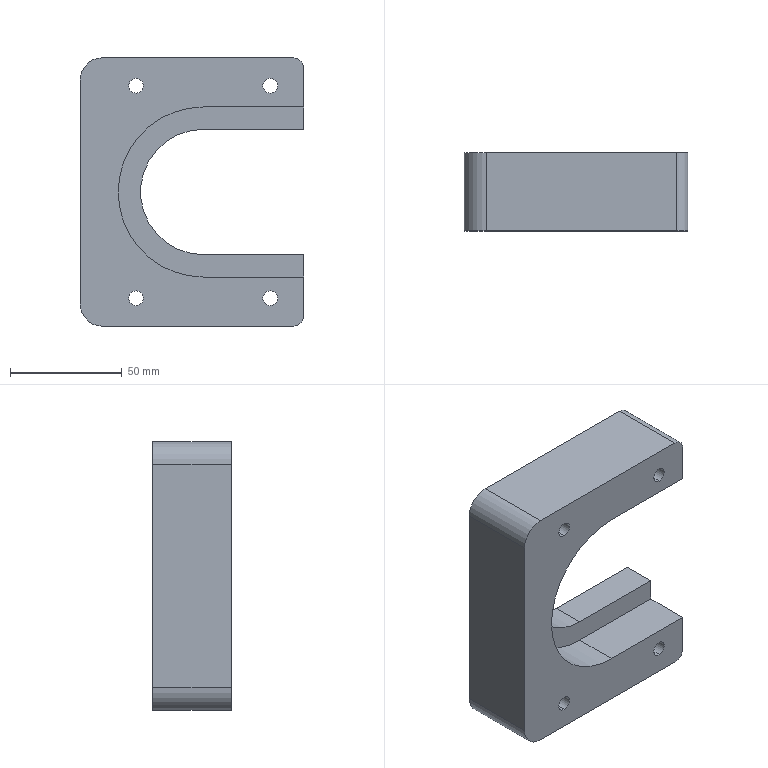Part | SolidWorks | features BaseBody 1 | 1 solid | 38 faces | box 100 x 35 x 120 mm | volume 241254 mm3 | cylinder 22 | plane 16 | commonest cylinder face diameters 6.6 x8 11 x8 10 x2 20 x2 56 x1 76 x1
STEP:
#1=CARTESIAN_POINT('',(-25.,28.2,-53.));
#2=VERTEX_POINT('',#1);
#3=CARTESIAN_POINT('',(-25.,28.2,-42.));
#4=VERTEX_POINT('',#3);
#5=CARTESIAN_POINT('',(-25.,28.2,-47.5));
#6=DIRECTION('',(0.,1.,0.));
#7=DIRECTION('',(0.,0.,1.));
#8=AXIS2_PLACEMENT_3D('',#5,#6,#7);
#9=CIRCLE('',#8,5.5);
#10=EDGE_CURVE('',#2,#4,#9,.T.);
#11=ORIENTED_EDGE('',*,*,#10,.F.);
#12=CARTESIAN_POINT('',(-25.,35.,-53.));
#13=VERTEX_POINT('',#12);
#14=CARTESIAN_POINT('',(-25.,35.,-53.));
#15=DIRECTION('',(0.,1.,0.));
#16=VECTOR('',#15,1000.);
#17=LINE('',#14,#16);
#18=EDGE_CURVE('',#2,#13,#17,.T.);
#19=ORIENTED_EDGE('',*,*,#18,.T.);
#20=CARTESIAN_POINT('',(-25.,35.,-42.));
#21=VERTEX_POINT('',#20);
#22=CARTESIAN_POINT('',(-25.,35.,-47.5));
#23=DIRECTION('',(0.,1.,0.));
#24=DIRECTION('',(0.,0.,1.));
#25=AXIS2_PLACEMENT_3D('',#22,#23,#24);
#26=CIRCLE('',#25,5.5);
#27=EDGE_CURVE('',#13,#21,#26,.T.);
#28=ORIENTED_EDGE('',*,*,#27,.T.);
#29=CARTESIAN_POINT('',(-25.,35.,-42.));
#30=DIRECTION('',(0.,1.,0.));
#31=VECTOR('',#30,1000.);
#32=LINE('',#29,#31);
#33=EDGE_CURVE('',#4,#21,#32,.T.);
#34=ORIENTED_EDGE('',*,*,#33,.F.);
#35=EDGE_LOOP('',(#11,#19,#28,#34));
#36=FACE_OUTER_BOUND('',#35,.T.);
#37=CARTESIAN_POINT('',(-25.,35.,-47.5));
#38=DIRECTION('',(0.,1.,0.));
#39=DIRECTION('',(0.,0.,1.));
#40=AXIS2_PLACEMENT_3D('',#37,#38,#39);
#41=CYLINDRICAL_SURFACE('',#40,5.5);
#42=ADVANCED_FACE('',(#36),#41,.F.);
#43=CARTESIAN_POINT('',(-25.,0.,-50.8));
#44=VERTEX_POINT('',#43);
#45=CARTESIAN_POINT('',(-25.,0.,-44.2));
#46=VERTEX_POINT('',#45);
#47=CARTESIAN_POINT('',(-25.,0.,-47.5));
#48=DIRECTION('',(0.,1.,0.));
#49=DIRECTION('',(0.,0.,1.));
#50=AXIS2_PLACEMENT_3D('',#47,#48,#49);
#51=CIRCLE('',#50,3.3);
#52=EDGE_CURVE('',#44,#46,#51,.T.);
#53=ORIENTED_EDGE('',*,*,#52,.F.);
#54=CARTESIAN_POINT('',(-25.,28.2,-50.8));
#55=VERTEX_POINT('',#54);
#56=CARTESIAN_POINT('',(-25.,35.,-50.8));
#57=DIRECTION('',(0.,1.,0.));
#58=VECTOR('',#57,1000.);
#59=LINE('',#56,#58);
#60=EDGE_CURVE('',#44,#55,#59,.T.);
#61=ORIENTED_EDGE('',*,*,#60,.T.);
#62=CARTESIAN_POINT('',(-25.,28.2,-44.2));
#63=VERTEX_POINT('',#62);
#64=CARTESIAN_POINT('',(-25.,28.2,-47.5));
#65=DIRECTION('',(0.,1.,0.));
#66=DIRECTION('',(0.,0.,1.));
#67=AXIS2_PLACEMENT_3D('',#64,#65,#66);
#68=CIRCLE('',#67,3.3);
#69=EDGE_CURVE('',#55,#63,#68,.T.);
#70=ORIENTED_EDGE('',*,*,#69,.T.);
#71=CARTESIAN_POINT('',(-25.,35.,-44.2));
#72=DIRECTION('',(0.,1.,0.));
#73=VECTOR('',#72,1000.);
#74=LINE('',#71,#73);
#75=EDGE_CURVE('',#46,#63,#74,.T.);
#76=ORIENTED_EDGE('',*,*,#75,.F.);
#77=EDGE_LOOP('',(#53,#61,#70,#76));
#78=FACE_OUTER_BOUND('',#77,.T.);
#79=CARTESIAN_POINT('',(-25.,35.,-47.5));
#80=DIRECTION('',(0.,1.,0.));
#81=DIRECTION('',(0.,0.,1.));
#82=AXIS2_PLACEMENT_3D('',#79,#80,#81);
#83=CYLINDRICAL_SURFACE('',#82,3.3);
#84=ADVANCED_FACE('',(#78),#83,.F.);
#85=CARTESIAN_POINT('',(35.,28.2,-53.));
#86=VERTEX_POINT('',#85);
#87=CARTESIAN_POINT('',(35.,28.2,-42.));
#88=VERTEX_POINT('',#87);
#89=CARTESIAN_POINT('',(35.,28.2,-47.5));
#90=DIRECTION('',(0.,1.,0.));
#91=DIRECTION('',(0.,0.,1.));
#92=AXIS2_PLACEMENT_3D('',#89,#90,#91);
#93=CIRCLE('',#92,5.5);
#94=EDGE_CURVE('',#86,#88,#93,.T.);
#95=ORIENTED_EDGE('',*,*,#94,.F.);
#96=CARTESIAN_POINT('',(35.,35.,-53.));
#97=VERTEX_POINT('',#96);
#98=CARTESIAN_POINT('',(35.,35.,-53.));
#99=DIRECTION('',(0.,1.,0.));
#100=VECTOR('',#99,1000.);
#101=LINE('',#98,#100);
#102=EDGE_CURVE('',#86,#97,#101,.T.);
#103=ORIENTED_EDGE('',*,*,#102,.T.);
#104=CARTESIAN_POINT('',(35.,35.,-42.));
#105=VERTEX_POINT('',#104);
#106=CARTESIAN_POINT('',(35.,35.,-47.5));
#107=DIRECTION('',(0.,1.,0.));
#108=DIRECTION('',(0.,0.,1.));
#109=AXIS2_PLACEMENT_3D('',#106,#107,#108);
#110=CIRCLE('',#109,5.5);
#111=EDGE_CURVE('',#97,#105,#110,.T.);
#112=ORIENTED_EDGE('',*,*,#111,.T.);
#113=CARTESIAN_POINT('',(35.,35.,-42.));
#114=DIRECTION('',(0.,1.,0.));
#115=VECTOR('',#114,1000.);
#116=LINE('',#113,#115);
#117=EDGE_CURVE('',#88,#105,#116,.T.);
#118=ORIENTED_EDGE('',*,*,#117,.F.);
#119=EDGE_LOOP('',(#95,#103,#112,#118));
#120=FACE_OUTER_BOUND('',#119,.T.);
#121=CARTESIAN_POINT('',(35.,35.,-47.5));
#122=DIRECTION('',(0.,1.,0.));
#123=DIRECTION('',(0.,0.,1.));
#124=AXIS2_PLACEMENT_3D('',#121,#122,#123);
#125=CYLINDRICAL_SURFACE('',#124,5.5);
#126=ADVANCED_FACE('',(#120),#125,.F.);
#127=CARTESIAN_POINT('',(35.,0.,-50.8));
#128=VERTEX_POINT('',#127);
#129=CARTESIAN_POINT('',(35.,0.,-44.2));
#130=VERTEX_POINT('',#129);
#131=CARTESIAN_POINT('',(35.,0.,-47.5));
#132=DIRECTION('',(0.,1.,0.));
#133=DIRECTION('',(0.,0.,1.));
#134=AXIS2_PLACEMENT_3D('',#131,#132,#133);
#135=CIRCLE('',#134,3.3);
#136=EDGE_CURVE('',#128,#130,#135,.T.);
#137=ORIENTED_EDGE('',*,*,#136,.F.);
#138=CARTESIAN_POINT('',(35.,28.2,-50.8));
#139=VERTEX_POINT('',#138);
#140=CARTESIAN_POINT('',(35.,35.,-50.8));
#141=DIRECTION('',(0.,1.,0.));
#142=VECTOR('',#141,1000.);
#143=LINE('',#140,#142);
#144=EDGE_CURVE('',#128,#139,#143,.T.);
#145=ORIENTED_EDGE('',*,*,#144,.T.);
#146=CARTESIAN_POINT('',(35.,28.2,-44.2));
#147=VERTEX_POINT('',#146);
#148=CARTESIAN_POINT('',(35.,28.2,-47.5));
#149=DIRECTION('',(0.,1.,0.));
#150=DIRECTION('',(0.,0.,1.));
#151=AXIS2_PLACEMENT_3D('',#148,#149,#150);
#152=CIRCLE('',#151,3.3);
#153=EDGE_CURVE('',#139,#147,#152,.T.);
#154=ORIENTED_EDGE('',*,*,#153,.T.);
#155=CARTESIAN_POINT('',(35.,35.,-44.2));
#156=DIRECTION('',(0.,1.,0.));
#157=VECTOR('',#156,1000.);
#158=LINE('',#155,#157);
#159=EDGE_CURVE('',#130,#147,#158,.T.);
#160=ORIENTED_EDGE('',*,*,#159,.F.);
#161=EDGE_LOOP('',(#137,#145,#154,#160));
#162=FACE_OUTER_BOUND('',#161,.T.);
#163=CARTESIAN_POINT('',(35.,35.,-47.5));
#164=DIRECTION('',(0.,1.,0.));
#165=DIRECTION('',(0.,0.,1.));
#166=AXIS2_PLACEMENT_3D('',#163,#164,#165);
#167=CYLINDRICAL_SURFACE('',#166,3.3);
#168=ADVANCED_FACE('',(#162),#167,.F.);
#169=CARTESIAN_POINT('',(35.,28.2,42.));
#170=VERTEX_POINT('',#169);
#171=CARTESIAN_POINT('',(35.,28.2,53.));
#172=VERTEX_POINT('',#171);
#173=CARTESIAN_POINT('',(35.,28.2,47.5));
#174=DIRECTION('',(0.,1.,0.));
#175=DIRECTION('',(0.,0.,1.));
#176=AXIS2_PLACEMENT_3D('',#173,#174,#175);
#177=CIRCLE('',#176,5.5);
#178=EDGE_CURVE('',#170,#172,#177,.T.);
#179=ORIENTED_EDGE('',*,*,#178,.F.);
#180=CARTESIAN_POINT('',(35.,35.,42.));
#181=VERTEX_POINT('',#180);
#182=CARTESIAN_POINT('',(35.,35.,42.));
#183=DIRECTION('',(0.,1.,0.));
#184=VECTOR('',#183,1000.);
#185=LINE('',#182,#184);
#186=EDGE_CURVE('',#170,#181,#185,.T.);
#187=ORIENTED_EDGE('',*,*,#186,.T.);
#188=CARTESIAN_POINT('',(35.,35.,53.));
#189=VERTEX_POINT('',#188);
#190=CARTESIAN_POINT('',(35.,35.,47.5));
#191=DIRECTION('',(0.,1.,0.));
#192=DIRECTION('',(0.,0.,1.));
#193=AXIS2_PLACEMENT_3D('',#190,#191,#192);
#194=CIRCLE('',#193,5.5);
#195=EDGE_CURVE('',#181,#189,#194,.T.);
#196=ORIENTED_EDGE('',*,*,#195,.T.);
#197=CARTESIAN_POINT('',(35.,35.,53.));
#198=DIRECTION('',(0.,1.,0.));
#199=VECTOR('',#198,1000.);
#200=LINE('',#197,#199);
#201=EDGE_CURVE('',#172,#189,#200,.T.);
#202=ORIENTED_EDGE('',*,*,#201,.F.);
#203=EDGE_LOOP('',(#179,#187,#196,#202));
#204=FACE_OUTER_BOUND('',#203,.T.);
#205=CARTESIAN_POINT('',(35.,35.,47.5));
#206=DIRECTION('',(0.,1.,0.));
#207=DIRECTION('',(0.,0.,1.));
#208=AXIS2_PLACEMENT_3D('',#205,#206,#207);
#209=CYLINDRICAL_SURFACE('',#208,5.5);
#210=ADVANCED_FACE('',(#204),#209,.F.);
#211=CARTESIAN_POINT('',(35.,0.,44.2));
#212=VERTEX_POINT('',#211);
#213=CARTESIAN_POINT('',(35.,0.,50.8));
#214=VERTEX_POINT('',#213);
#215=CARTESIAN_POINT('',(35.,0.,47.5));
#216=DIRECTION('',(0.,1.,0.));
#217=DIRECTION('',(0.,0.,1.));
#218=AXIS2_PLACEMENT_3D('',#215,#216,#217);
#219=CIRCLE('',#218,3.3);
#220=EDGE_CURVE('',#212,#214,#219,.T.);
#221=ORIENTED_EDGE('',*,*,#220,.F.);
#222=CARTESIAN_POINT('',(35.,28.2,44.2));
#223=VERTEX_POINT('',#222);
#224=CARTESIAN_POINT('',(35.,35.,44.2));
#225=DIRECTION('',(0.,1.,0.));
#226=VECTOR('',#225,1000.);
#227=LINE('',#224,#226);
#228=EDGE_CURVE('',#212,#223,#227,.T.);
#229=ORIENTED_EDGE('',*,*,#228,.T.);
#230=CARTESIAN_POINT('',(35.,28.2,50.8));
#231=VERTEX_POINT('',#230);
#232=CARTESIAN_POINT('',(35.,28.2,47.5));
#233=DIRECTION('',(0.,1.,0.));
#234=DIRECTION('',(0.,0.,1.));
#235=AXIS2_PLACEMENT_3D('',#232,#233,#234);
#236=CIRCLE('',#235,3.3);
#237=EDGE_CURVE('',#223,#231,#236,.T.);
#238=ORIENTED_EDGE('',*,*,#237,.T.);
#239=CARTESIAN_POINT('',(35.,35.,50.8));
#240=DIRECTION('',(0.,1.,0.));
#241=VECTOR('',#240,1000.);
#242=LINE('',#239,#241);
#243=EDGE_CURVE('',#214,#231,#242,.T.);
#244=ORIENTED_EDGE('',*,*,#243,.F.);
#245=EDGE_LOOP('',(#221,#229,#238,#244));
#246=FACE_OUTER_BOUND('',#245,.T.);
#247=CARTESIAN_POINT('',(35.,35.,47.5));
#248=DIRECTION('',(0.,1.,0.));
#249=DIRECTION('',(0.,0.,1.));
#250=AXIS2_PLACEMENT_3D('',#247,#248,#249);
#251=CYLINDRICAL_SURFACE('',#250,3.3);
#252=ADVANCED_FACE('',(#246),#251,.F.);
#253=CARTESIAN_POINT('',(-25.,28.2,42.));
#254=VERTEX_POINT('',#253);
#255=CARTESIAN_POINT('',(-25.,28.2,53.));
#256=VERTEX_POINT('',#255);
#257=CARTESIAN_POINT('',(-25.,28.2,47.5));
#258=DIRECTION('',(0.,1.,0.));
#259=DIRECTION('',(0.,0.,1.));
#260=AXIS2_PLACEMENT_3D('',#257,#258,#259);
#261=CIRCLE('',#260,5.5);
#262=EDGE_CURVE('',#254,#256,#261,.T.);
#263=ORIENTED_EDGE('',*,*,#262,.F.);
#264=CARTESIAN_POINT('',(-25.,35.,42.));
#265=VERTEX_POINT('',#264);
#266=CARTESIAN_POINT('',(-25.,35.,42.));
#267=DIRECTION('',(0.,1.,0.));
#268=VECTOR('',#267,1000.);
#269=LINE('',#266,#268);
#270=EDGE_CURVE('',#254,#265,#269,.T.);
#271=ORIENTED_EDGE('',*,*,#270,.T.);
#272=CARTESIAN_POINT('',(-25.,35.,53.));
#273=VERTEX_POINT('',#272);
#274=CARTESIAN_POINT('',(-25.,35.,47.5));
#275=DIRECTION('',(0.,1.,0.));
#276=DIRECTION('',(0.,0.,1.));
#277=AXIS2_PLACEMENT_3D('',#274,#275,#276);
#278=CIRCLE('',#277,5.5);
#279=EDGE_CURVE('',#265,#273,#278,.T.);
#280=ORIENTED_EDGE('',*,*,#279,.T.);
#281=CARTESIAN_POINT('',(-25.,35.,53.));
#282=DIRECTION('',(0.,1.,0.));
#283=VECTOR('',#282,1000.);
#284=LINE('',#281,#283);
#285=EDGE_CURVE('',#256,#273,#284,.T.);
#286=ORIENTED_EDGE('',*,*,#285,.F.);
#287=EDGE_LOOP('',(#263,#271,#280,#286));
#288=FACE_OUTER_BOUND('',#287,.T.);
#289=CARTESIAN_POINT('',(-25.,35.,47.5));
#290=DIRECTION('',(0.,1.,0.));
#291=DIRECTION('',(0.,0.,1.));
#292=AXIS2_PLACEMENT_3D('',#289,#290,#291);
#293=CYLINDRICAL_SURFACE('',#292,5.5);
#294=ADVANCED_FACE('',(#288),#293,.F.);
#295=CARTESIAN_POINT('',(-25.,0.,44.2));
#296=VERTEX_POINT('',#295);
#297=CARTESIAN_POINT('',(-25.,0.,50.8));
#298=VERTEX_POINT('',#297);
#299=CARTESIAN_POINT('',(-25.,0.,47.5));
#300=DIRECTION('',(0.,1.,0.));
#301=DIRECTION('',(0.,0.,1.));
#302=AXIS2_PLACEMENT_3D('',#299,#300,#301);
#303=CIRCLE('',#302,3.3);
#304=EDGE_CURVE('',#296,#298,#303,.T.);
#305=ORIENTED_EDGE('',*,*,#304,.F.);
#306=CARTESIAN_POINT('',(-25.,28.2,44.2));
#307=VERTEX_POINT('',#306);
#308=CARTESIAN_POINT('',(-25.,35.,44.2));
#309=DIRECTION('',(0.,1.,0.));
#310=VECTOR('',#309,1000.);
#311=LINE('',#308,#310);
#312=EDGE_CURVE('',#296,#307,#311,.T.);
#313=ORIENTED_EDGE('',*,*,#312,.T.);
#314=CARTESIAN_POINT('',(-25.,28.2,50.8));
#315=VERTEX_POINT('',#314);
#316=CARTESIAN_POINT('',(-25.,28.2,47.5));
#317=DIRECTION('',(0.,1.,0.));
#318=DIRECTION('',(0.,0.,1.));
#319=AXIS2_PLACEMENT_3D('',#316,#317,#318);
#320=CIRCLE('',#319,3.3);
#321=EDGE_CURVE('',#307,#315,#320,.T.);
#322=ORIENTED_EDGE('',*,*,#321,.T.);
#323=CARTESIAN_POINT('',(-25.,35.,50.8));
#324=DIRECTION('',(0.,1.,0.));
#325=VECTOR('',#324,1000.);
#326=LINE('',#323,#325);
#327=EDGE_CURVE('',#298,#315,#326,.T.);
#328=ORIENTED_EDGE('',*,*,#327,.F.);
#329=EDGE_LOOP('',(#305,#313,#322,#328));
#330=FACE_OUTER_BOUND('',#329,.T.);
#331=CARTESIAN_POINT('',(-25.,35.,47.5));
#332=DIRECTION('',(0.,1.,0.));
#333=DIRECTION('',(0.,0.,1.));
#334=AXIS2_PLACEMENT_3D('',#331,#332,#333);
#335=CYLINDRICAL_SURFACE('',#334,3.3);
#336=ADVANCED_FACE('',(#330),#335,.F.);
#337=CARTESIAN_POINT('',(-25.,28.2,-47.5));
#338=DIRECTION('',(0.,1.,0.));
#339=DIRECTION('',(0.,0.,1.));
#340=AXIS2_PLACEMENT_3D('',#337,#338,#339);
#341=CIRCLE('',#340,3.3);
#342=EDGE_CURVE('',#63,#55,#341,.T.);
#343=ORIENTED_EDGE('',*,*,#342,.F.);
#344=ORIENTED_EDGE('',*,*,#69,.F.);
#345=EDGE_LOOP('',(#343,#344));
#346=FACE_BOUND('',#345,.T.);
#347=CARTESIAN_POINT('',(-25.,28.2,-47.5));
#348=DIRECTION('',(0.,1.,0.));
#349=DIRECTION('',(0.,0.,1.));
#350=AXIS2_PLACEMENT_3D('',#347,#348,#349);
#351=CIRCLE('',#350,5.5);
#352=EDGE_CURVE('',#4,#2,#351,.T.);
#353=ORIENTED_EDGE('',*,*,#352,.T.);
#354=ORIENTED_EDGE('',*,*,#10,.T.);
#355=EDGE_LOOP('',(#353,#354));
#356=FACE_OUTER_BOUND('',#355,.T.);
#357=CARTESIAN_POINT('',(-21.7,28.2,-47.5));
#358=DIRECTION('',(0.,-1.,0.));
#359=DIRECTION('',(0.,0.,-1.));
#360=AXIS2_PLACEMENT_3D('',#357,#358,#359);
#361=PLANE('',#360);
#362=ADVANCED_FACE('',(#346,#356),#361,.F.);
#363=CARTESIAN_POINT('',(35.,28.2,-47.5));
#364=DIRECTION('',(0.,1.,0.));
#365=DIRECTION('',(0.,0.,1.));
#366=AXIS2_PLACEMENT_3D('',#363,#364,#365);
#367=CIRCLE('',#366,3.3);
#368=EDGE_CURVE('',#147,#139,#367,.T.);
#369=ORIENTED_EDGE('',*,*,#368,.F.);
#370=ORIENTED_EDGE('',*,*,#153,.F.);
#371=EDGE_LOOP('',(#369,#370));
#372=FACE_BOUND('',#371,.T.);
#373=CARTESIAN_POINT('',(35.,28.2,-47.5));
#374=DIRECTION('',(0.,1.,0.));
#375=DIRECTION('',(0.,0.,1.));
#376=AXIS2_PLACEMENT_3D('',#373,#374,#375);
#377=CIRCLE('',#376,5.5);
#378=EDGE_CURVE('',#88,#86,#377,.T.);
#379=ORIENTED_EDGE('',*,*,#378,.T.);
#380=ORIENTED_EDGE('',*,*,#94,.T.);
#381=EDGE_LOOP('',(#379,#380));
#382=FACE_OUTER_BOUND('',#381,.T.);
#383=CARTESIAN_POINT('',(38.3,28.2,-47.5));
#384=DIRECTION('',(0.,-1.,0.));
#385=DIRECTION('',(0.,0.,-1.));
#386=AXIS2_PLACEMENT_3D('',#383,#384,#385);
#387=PLANE('',#386);
#388=ADVANCED_FACE('',(#372,#382),#387,.F.);
#389=CARTESIAN_POINT('',(35.,28.2,47.5));
#390=DIRECTION('',(0.,1.,0.));
#391=DIRECTION('',(0.,0.,1.));
#392=AXIS2_PLACEMENT_3D('',#389,#390,#391);
#393=CIRCLE('',#392,3.3);
#394=EDGE_CURVE('',#231,#223,#393,.T.);
#395=ORIENTED_EDGE('',*,*,#394,.F.);
#396=ORIENTED_EDGE('',*,*,#237,.F.);
#397=EDGE_LOOP('',(#395,#396));
#398=FACE_BOUND('',#397,.T.);
#399=CARTESIAN_POINT('',(35.,28.2,47.5));
#400=DIRECTION('',(0.,1.,0.));
#401=DIRECTION('',(0.,0.,1.));
#402=AXIS2_PLACEMENT_3D('',#399,#400,#401);
#403=CIRCLE('',#402,5.5);
#404=EDGE_CURVE('',#172,#170,#403,.T.);
#405=ORIENTED_EDGE('',*,*,#404,.T.);
#406=ORIENTED_EDGE('',*,*,#178,.T.);
#407=EDGE_LOOP('',(#405,#406));
#408=FACE_OUTER_BOUND('',#407,.T.);
#409=CARTESIAN_POINT('',(38.3,28.2,47.5));
#410=DIRECTION('',(0.,-1.,0.));
#411=DIRECTION('',(0.,0.,-1.));
#412=AXIS2_PLACEMENT_3D('',#409,#410,#411);
#413=PLANE('',#412);
#414=ADVANCED_FACE('',(#398,#408),#413,.F.);
#415=CARTESIAN_POINT('',(-25.,28.2,47.5));
#416=DIRECTION('',(0.,1.,0.));
#417=DIRECTION('',(0.,0.,1.));
#418=AXIS2_PLACEMENT_3D('',#415,#416,#417);
#419=CIRCLE('',#418,3.3);
#420=EDGE_CURVE('',#315,#307,#419,.T.);
#421=ORIENTED_EDGE('',*,*,#420,.F.);
#422=ORIENTED_EDGE('',*,*,#321,.F.);
#423=EDGE_LOOP('',(#421,#422));
#424=FACE_BOUND('',#423,.T.);
#425=CARTESIAN_POINT('',(-25.,28.2,47.5));
#426=DIRECTION('',(0.,1.,0.));
#427=DIRECTION('',(0.,0.,1.));
#428=AXIS2_PLACEMENT_3D('',#425,#426,#427);
#429=CIRCLE('',#428,5.5);
#430=EDGE_CURVE('',#256,#254,#429,.T.);
#431=ORIENTED_EDGE('',*,*,#430,.T.);
#432=ORIENTED_EDGE('',*,*,#262,.T.);
#433=EDGE_LOOP('',(#431,#432));
#434=FACE_OUTER_BOUND('',#433,.T.);
#435=CARTESIAN_POINT('',(-21.7,28.2,47.5));
#436=DIRECTION('',(0.,-1.,0.));
#437=DIRECTION('',(0.,0.,-1.));
#438=AXIS2_PLACEMENT_3D('',#435,#436,#437);
#439=PLANE('',#438);
#440=ADVANCED_FACE('',(#424,#434),#439,.F.);
#441=CARTESIAN_POINT('',(45.,35.,60.));
#442=VERTEX_POINT('',#441);
#443=CARTESIAN_POINT('',(50.,35.,55.));
#444=VERTEX_POINT('',#443);
#445=CARTESIAN_POINT('',(45.,35.,55.));
#446=DIRECTION('',(0.,1.,0.));
#447=DIRECTION('',(0.,0.,1.));
#448=AXIS2_PLACEMENT_3D('',#445,#446,#447);
#449=CIRCLE('',#448,5.);
#450=EDGE_CURVE('',#442,#444,#449,.T.);
#451=ORIENTED_EDGE('',*,*,#450,.F.);
#452=CARTESIAN_POINT('',(45.,0.,60.));
#453=VERTEX_POINT('',#452);
#454=CARTESIAN_POINT('',(45.,35.,60.));
#455=DIRECTION('',(0.,1.,0.));
#456=VECTOR('',#455,1000.);
#457=LINE('',#454,#456);
#458=EDGE_CURVE('',#453,#442,#457,.T.);
#459=ORIENTED_EDGE('',*,*,#458,.F.);
#460=CARTESIAN_POINT('',(50.,0.,55.));
#461=VERTEX_POINT('',#460);
#462=CARTESIAN_POINT('',(45.,0.,55.));
#463=DIRECTION('',(0.,-1.,0.));
#464=DIRECTION('',(0.,0.,1.));
#465=AXIS2_PLACEMENT_3D('',#462,#463,#464);
#466=CIRCLE('',#465,5.);
#467=EDGE_CURVE('',#461,#453,#466,.T.);
#468=ORIENTED_EDGE('',*,*,#467,.F.);
#469=CARTESIAN_POINT('',(50.,35.,55.));
#470=DIRECTION('',(0.,-1.,0.));
#471=VECTOR('',#470,1000.);
#472=LINE('',#469,#471);
#473=EDGE_CURVE('',#444,#461,#472,.T.);
#474=ORIENTED_EDGE('',*,*,#473,.F.);
#475=EDGE_LOOP('',(#451,#459,#468,#474));
#476=FACE_OUTER_BOUND('',#475,.T.);
#477=CARTESIAN_POINT('',(45.,35.,55.));
#478=DIRECTION('',(0.,-1.,0.));
#479=DIRECTION('',(0.,0.,-1.));
#480=AXIS2_PLACEMENT_3D('',#477,#478,#479);
#481=CYLINDRICAL_SURFACE('',#480,5.);
#482=ADVANCED_FACE('',(#476),#481,.T.);
#483=CARTESIAN_POINT('',(50.,35.,-55.));
#484=VERTEX_POINT('',#483);
#485=CARTESIAN_POINT('',(45.,35.,-60.));
#486=VERTEX_POINT('',#485);
#487=CARTESIAN_POINT('',(45.,35.,-55.));
#488=DIRECTION('',(0.,1.,0.));
#489=DIRECTION('',(0.,0.,1.));
#490=AXIS2_PLACEMENT_3D('',#487,#488,#489);
#491=CIRCLE('',#490,5.);
#492=EDGE_CURVE('',#484,#486,#491,.T.);
#493=ORIENTED_EDGE('',*,*,#492,.F.);
#494=CARTESIAN_POINT('',(50.,0.,-55.));
#495=VERTEX_POINT('',#494);
#496=CARTESIAN_POINT('',(50.,35.,-55.));
#497=DIRECTION('',(0.,1.,0.));
#498=VECTOR('',#497,1000.);
#499=LINE('',#496,#498);
#500=EDGE_CURVE('',#495,#484,#499,.T.);
#501=ORIENTED_EDGE('',*,*,#500,.F.);
#502=CARTESIAN_POINT('',(45.,0.,-60.));
#503=VERTEX_POINT('',#502);
#504=CARTESIAN_POINT('',(45.,0.,-55.));
#505=DIRECTION('',(0.,-1.,0.));
#506=DIRECTION('',(0.,0.,1.));
#507=AXIS2_PLACEMENT_3D('',#504,#505,#506);
#508=CIRCLE('',#507,5.);
#509=EDGE_CURVE('',#503,#495,#508,.T.);
#510=ORIENTED_EDGE('',*,*,#509,.F.);
#511=CARTESIAN_POINT('',(45.,35.,-60.));
#512=DIRECTION('',(0.,-1.,0.));
#513=VECTOR('',#512,1000.);
#514=LINE('',#511,#513);
#515=EDGE_CURVE('',#486,#503,#514,.T.);
#516=ORIENTED_EDGE('',*,*,#515,.F.);
#517=EDGE_LOOP('',(#493,#501,#510,#516));
#518=FACE_OUTER_BOUND('',#517,.T.);
#519=CARTESIAN_POINT('',(45.,35.,-55.));
#520=DIRECTION('',(0.,-1.,0.));
#521=DIRECTION('',(0.,0.,-1.));
#522=AXIS2_PLACEMENT_3D('',#519,#520,#521);
#523=CYLINDRICAL_SURFACE('',#522,5.);
#524=ADVANCED_FACE('',(#518),#523,.T.);
#525=CARTESIAN_POINT('',(-50.,35.,50.));
#526=VERTEX_POINT('',#525);
#527=CARTESIAN_POINT('',(-40.,35.,60.));
#528=VERTEX_POINT('',#527);
#529=CARTESIAN_POINT('',(-40.,35.,50.));
#530=DIRECTION('',(0.,1.,0.));
#531=DIRECTION('',(0.,0.,1.));
#532=AXIS2_PLACEMENT_3D('',#529,#530,#531);
#533=CIRCLE('',#532,10.);
#534=EDGE_CURVE('',#526,#528,#533,.T.);
#535=ORIENTED_EDGE('',*,*,#534,.F.);
#536=CARTESIAN_POINT('',(-50.,0.,50.));
#537=VERTEX_POINT('',#536);
#538=CARTESIAN_POINT('',(-50.,35.,50.));
#539=DIRECTION('',(0.,1.,0.));
#540=VECTOR('',#539,1000.);
#541=LINE('',#538,#540);
#542=EDGE_CURVE('',#537,#526,#541,.T.);
#543=ORIENTED_EDGE('',*,*,#542,.F.);
#544=CARTESIAN_POINT('',(-40.,0.,60.));
#545=VERTEX_POINT('',#544);
#546=CARTESIAN_POINT('',(-40.,0.,50.));
#547=DIRECTION('',(0.,-1.,0.));
#548=DIRECTION('',(0.,0.,1.));
#549=AXIS2_PLACEMENT_3D('',#546,#547,#548);
#550=CIRCLE('',#549,10.);
#551=EDGE_CURVE('',#545,#537,#550,.T.);
#552=ORIENTED_EDGE('',*,*,#551,.F.);
#553=CARTESIAN_POINT('',(-40.,35.,60.));
#554=DIRECTION('',(0.,-1.,0.));
#555=VECTOR('',#554,1000.);
#556=LINE('',#553,#555);
#557=EDGE_CURVE('',#528,#545,#556,.T.);
#558=ORIENTED_EDGE('',*,*,#557,.F.);
#559=EDGE_LOOP('',(#535,#543,#552,#558));
#560=FACE_OUTER_BOUND('',#559,.T.);
#561=CARTESIAN_POINT('',(-40.,35.,50.));
#562=DIRECTION('',(0.,-1.,0.));
#563=DIRECTION('',(0.,0.,-1.));
#564=AXIS2_PLACEMENT_3D('',#561,#562,#563);
#565=CYLINDRICAL_SURFACE('',#564,10.);
#566=ADVANCED_FACE('',(#560),#565,.T.);
#567=CARTESIAN_POINT('',(-40.,35.,-60.));
#568=VERTEX_POINT('',#567);
#569=CARTESIAN_POINT('',(-50.,35.,-50.));
#570=VERTEX_POINT('',#569);
#571=CARTESIAN_POINT('',(-40.,35.,-50.));
#572=DIRECTION('',(0.,1.,0.));
#573=DIRECTION('',(0.,0.,1.));
#574=AXIS2_PLACEMENT_3D('',#571,#572,#573);
#575=CIRCLE('',#574,10.);
#576=EDGE_CURVE('',#568,#570,#575,.T.);
#577=ORIENTED_EDGE('',*,*,#576,.F.);
#578=CARTESIAN_POINT('',(-40.,0.,-60.));
#579=VERTEX_POINT('',#578);
#580=CARTESIAN_POINT('',(-40.,35.,-60.));
#581=DIRECTION('',(0.,1.,0.));
#582=VECTOR('',#581,1000.);
#583=LINE('',#580,#582);
#584=EDGE_CURVE('',#579,#568,#583,.T.);
#585=ORIENTED_EDGE('',*,*,#584,.F.);
#586=CARTESIAN_POINT('',(-50.,0.,-50.));
#587=VERTEX_POINT('',#586);
#588=CARTESIAN_POINT('',(-40.,0.,-50.));
#589=DIRECTION('',(0.,-1.,0.));
#590=DIRECTION('',(0.,0.,1.));
#591=AXIS2_PLACEMENT_3D('',#588,#589,#590);
#592=CIRCLE('',#591,10.);
#593=EDGE_CURVE('',#587,#579,#592,.T.);
#594=ORIENTED_EDGE('',*,*,#593,.F.);
#595=CARTESIAN_POINT('',(-50.,35.,-50.));
#596=DIRECTION('',(0.,-1.,0.));
#597=VECTOR('',#596,1000.);
#598=LINE('',#595,#597);
#599=EDGE_CURVE('',#570,#587,#598,.T.);
#600=ORIENTED_EDGE('',*,*,#599,.F.);
#601=EDGE_LOOP('',(#577,#585,#594,#600));
#602=FACE_OUTER_BOUND('',#601,.T.);
#603=CARTESIAN_POINT('',(-40.,35.,-50.));
#604=DIRECTION('',(0.,-1.,0.));
#605=DIRECTION('',(0.,0.,-1.));
#606=AXIS2_PLACEMENT_3D('',#603,#604,#605);
#607=CYLINDRICAL_SURFACE('',#606,10.);
#608=ADVANCED_FACE('',(#602),#607,.T.);
#609=CARTESIAN_POINT('',(5.,0.,38.));
#610=VERTEX_POINT('',#609);
#611=CARTESIAN_POINT('',(5.,0.,-38.));
#612=VERTEX_POINT('',#611);
#613=CARTESIAN_POINT('',(5.,0.,0.));
#614=DIRECTION('',(0.,-1.,0.));
#615=DIRECTION('',(0.,0.,-1.));
#616=AXIS2_PLACEMENT_3D('',#613,#614,#615);
#617=CIRCLE('',#616,38.);
#618=EDGE_CURVE('',#610,#612,#617,.T.);
#619=ORIENTED_EDGE('',*,*,#618,.T.);
#620=CARTESIAN_POINT('',(5.,20.2,-38.));
#621=VERTEX_POINT('',#620);
#622=CARTESIAN_POINT('',(5.,20.2,-38.));
#623=DIRECTION('',(0.,-1.,0.));
#624=VECTOR('',#623,1000.);
#625=LINE('',#622,#624);
#626=EDGE_CURVE('',#621,#612,#625,.T.);
#627=ORIENTED_EDGE('',*,*,#626,.F.);
#628=CARTESIAN_POINT('',(5.,20.2,38.));
#629=VERTEX_POINT('',#628);
#630=CARTESIAN_POINT('',(5.,20.2,0.));
#631=DIRECTION('',(0.,-1.,0.));
#632=DIRECTION('',(0.,0.,-1.));
#633=AXIS2_PLACEMENT_3D('',#630,#631,#632);
#634=CIRCLE('',#633,38.);
#635=EDGE_CURVE('',#629,#621,#634,.T.);
#636=ORIENTED_EDGE('',*,*,#635,.F.);
#637=CARTESIAN_POINT('',(5.,20.2,38.));
#638=DIRECTION('',(0.,-1.,0.));
#639=VECTOR('',#638,1000.);
#640=LINE('',#637,#639);
#641=EDGE_CURVE('',#629,#610,#640,.T.);
#642=ORIENTED_EDGE('',*,*,#641,.T.);
#643=EDGE_LOOP('',(#619,#627,#636,#642));
#644=FACE_OUTER_BOUND('',#643,.T.);
#645=CARTESIAN_POINT('',(5.,20.2,0.));
#646=DIRECTION('',(0.,-1.,0.));
#647=DIRECTION('',(0.,0.,-1.));
#648=AXIS2_PLACEMENT_3D('',#645,#646,#647);
#649=CYLINDRICAL_SURFACE('',#648,38.);
#650=ADVANCED_FACE('',(#644),#649,.F.);
#651=CARTESIAN_POINT('',(50.,20.2,-38.));
#652=VERTEX_POINT('',#651);
#653=CARTESIAN_POINT('',(50.,20.2,-28.));
#654=VERTEX_POINT('',#653);
#655=CARTESIAN_POINT('',(50.,20.2,-60.));
#656=DIRECTION('',(0.,0.,1.));
#657=VECTOR('',#656,1000.);
#658=LINE('',#655,#657);
#659=EDGE_CURVE('',#652,#654,#658,.T.);
#660=ORIENTED_EDGE('',*,*,#659,.T.);
#661=CARTESIAN_POINT('',(5.,20.2,-28.));
#662=VERTEX_POINT('',#661);
#663=CARTESIAN_POINT('',(5.,20.2,-28.));
#664=DIRECTION('',(-1.,0.,0.));
#665=VECTOR('',#664,1000.);
#666=LINE('',#663,#665);
#667=EDGE_CURVE('',#654,#662,#666,.T.);
#668=ORIENTED_EDGE('',*,*,#667,.T.);
#669=CARTESIAN_POINT('',(5.,20.2,28.));
#670=VERTEX_POINT('',#669);
#671=CARTESIAN_POINT('',(5.,20.2,0.));
#672=DIRECTION('',(0.,1.,0.));
#673=DIRECTION('',(0.,0.,-1.));
#674=AXIS2_PLACEMENT_3D('',#671,#672,#673);
#675=CIRCLE('',#674,28.);
#676=EDGE_CURVE('',#662,#670,#675,.T.);
#677=ORIENTED_EDGE('',*,*,#676,.T.);
#678=CARTESIAN_POINT('',(50.,20.2,28.));
#679=VERTEX_POINT('',#678);
#680=CARTESIAN_POINT('',(5.,20.2,28.));
#681=DIRECTION('',(1.,0.,0.));
#682=VECTOR('',#681,1000.);
#683=LINE('',#680,#682);
#684=EDGE_CURVE('',#670,#679,#683,.T.);
#685=ORIENTED_EDGE('',*,*,#684,.T.);
#686=CARTESIAN_POINT('',(50.,20.2,38.));
#687=VERTEX_POINT('',#686);
#688=CARTESIAN_POINT('',(50.,20.2,-60.));
#689=DIRECTION('',(0.,0.,1.));
#690=VECTOR('',#689,1000.);
#691=LINE('',#688,#690);
#692=EDGE_CURVE('',#679,#687,#691,.T.);
#693=ORIENTED_EDGE('',*,*,#692,.T.);
#694=CARTESIAN_POINT('',(5.,20.2,38.));
#695=DIRECTION('',(-1.,0.,0.));
#696=VECTOR('',#695,1000.);
#697=LINE('',#694,#696);
#698=EDGE_CURVE('',#687,#629,#697,.T.);
#699=ORIENTED_EDGE('',*,*,#698,.T.);
#700=ORIENTED_EDGE('',*,*,#635,.T.);
#701=CARTESIAN_POINT('',(5.,20.2,-38.));
#702=DIRECTION('',(1.,0.,0.));
#703=VECTOR('',#702,1000.);
#704=LINE('',#701,#703);
#705=EDGE_CURVE('',#621,#652,#704,.T.);
#706=ORIENTED_EDGE('',*,*,#705,.T.);
#707=EDGE_LOOP('',(#660,#668,#677,#685,#693,#699,#700,#706));
#708=FACE_OUTER_BOUND('',#707,.T.);
#709=CARTESIAN_POINT('',(5.,20.2,0.));
#710=DIRECTION('',(0.,-1.,0.));
#711=DIRECTION('',(0.,0.,-1.));
#712=AXIS2_PLACEMENT_3D('',#709,#710,#711);
#713=PLANE('',#712);
#714=ADVANCED_FACE('',(#708),#713,.T.);
#715=ORIENTED_EDGE('',*,*,#705,.F.);
#716=ORIENTED_EDGE('',*,*,#626,.T.);
#717=CARTESIAN_POINT('',(50.,0.,-38.));
#718=VERTEX_POINT('',#717);
#719=CARTESIAN_POINT('',(5.,0.,-38.));
#720=DIRECTION('',(1.,0.,0.));
#721=VECTOR('',#720,1000.);
#722=LINE('',#719,#721);
#723=EDGE_CURVE('',#612,#718,#722,.T.);
#724=ORIENTED_EDGE('',*,*,#723,.T.);
#725=CARTESIAN_POINT('',(50.,35.,-38.));
#726=DIRECTION('',(0.,-1.,0.));
#727=VECTOR('',#726,1000.);
#728=LINE('',#725,#727);
#729=EDGE_CURVE('',#652,#718,#728,.T.);
#730=ORIENTED_EDGE('',*,*,#729,.F.);
#731=EDGE_LOOP('',(#715,#716,#724,#730));
#732=FACE_OUTER_BOUND('',#731,.T.);
#733=CARTESIAN_POINT('',(5.,20.2,-38.));
#734=DIRECTION('',(0.,0.,-1.));
#735=DIRECTION('',(0.,-1.,0.));
#736=AXIS2_PLACEMENT_3D('',#733,#734,#735);
#737=PLANE('',#736);
#738=ADVANCED_FACE('',(#732),#737,.F.);
#739=CARTESIAN_POINT('',(50.,0.,38.));
#740=VERTEX_POINT('',#739);
#741=CARTESIAN_POINT('',(5.,0.,38.));
#742=DIRECTION('',(-1.,0.,0.));
#743=VECTOR('',#742,1000.);
#744=LINE('',#741,#743);
#745=EDGE_CURVE('',#740,#610,#744,.T.);
#746=ORIENTED_EDGE('',*,*,#745,.T.);
#747=ORIENTED_EDGE('',*,*,#641,.F.);
#748=ORIENTED_EDGE('',*,*,#698,.F.);
#749=CARTESIAN_POINT('',(50.,35.,38.));
#750=DIRECTION('',(0.,1.,0.));
#751=VECTOR('',#750,1000.);
#752=LINE('',#749,#751);
#753=EDGE_CURVE('',#740,#687,#752,.T.);
#754=ORIENTED_EDGE('',*,*,#753,.F.);
#755=EDGE_LOOP('',(#746,#747,#748,#754));
#756=FACE_OUTER_BOUND('',#755,.T.);
#757=CARTESIAN_POINT('',(5.,20.2,38.));
#758=DIRECTION('',(0.,0.,1.));
#759=DIRECTION('',(1.,0.,0.));
#760=AXIS2_PLACEMENT_3D('',#757,#758,#759);
#761=PLANE('',#760);
#762=ADVANCED_FACE('',(#756),#761,.F.);
#763=CARTESIAN_POINT('',(-25.,0.,47.5));
#764=DIRECTION('',(0.,1.,0.));
#765=DIRECTION('',(0.,0.,1.));
#766=AXIS2_PLACEMENT_3D('',#763,#764,#765);
#767=CIRCLE('',#766,3.3);
#768=EDGE_CURVE('',#298,#296,#767,.T.);
#769=ORIENTED_EDGE('',*,*,#768,.T.);
#770=ORIENTED_EDGE('',*,*,#304,.T.);
#771=EDGE_LOOP('',(#769,#770));
#772=FACE_BOUND('',#771,.T.);
#773=CARTESIAN_POINT('',(35.,0.,47.5));
#774=DIRECTION('',(0.,1.,0.));
#775=DIRECTION('',(0.,0.,1.));
#776=AXIS2_PLACEMENT_3D('',#773,#774,#775);
#777=CIRCLE('',#776,3.3);
#778=EDGE_CURVE('',#214,#212,#777,.T.);
#779=ORIENTED_EDGE('',*,*,#778,.T.);
#780=ORIENTED_EDGE('',*,*,#220,.T.);
#781=EDGE_LOOP('',(#779,#780));
#782=FACE_BOUND('',#781,.T.);
#783=CARTESIAN_POINT('',(35.,0.,-47.5));
#784=DIRECTION('',(0.,1.,0.));
#785=DIRECTION('',(0.,0.,1.));
#786=AXIS2_PLACEMENT_3D('',#783,#784,#785);
#787=CIRCLE('',#786,3.3);
#788=EDGE_CURVE('',#130,#128,#787,.T.);
#789=ORIENTED_EDGE('',*,*,#788,.T.);
#790=ORIENTED_EDGE('',*,*,#136,.T.);
#791=EDGE_LOOP('',(#789,#790));
#792=FACE_BOUND('',#791,.T.);
#793=CARTESIAN_POINT('',(-25.,0.,-47.5));
#794=DIRECTION('',(0.,1.,0.));
#795=DIRECTION('',(0.,0.,1.));
#796=AXIS2_PLACEMENT_3D('',#793,#794,#795);
#797=CIRCLE('',#796,3.3);
#798=EDGE_CURVE('',#46,#44,#797,.T.);
#799=ORIENTED_EDGE('',*,*,#798,.T.);
#800=ORIENTED_EDGE('',*,*,#52,.T.);
#801=EDGE_LOOP('',(#799,#800));
#802=FACE_BOUND('',#801,.T.);
#803=CARTESIAN_POINT('',(-50.,0.,-60.));
#804=DIRECTION('',(-1.,0.,0.));
#805=VECTOR('',#804,1000.);
#806=LINE('',#803,#805);
#807=EDGE_CURVE('',#503,#579,#806,.T.);
#808=ORIENTED_EDGE('',*,*,#807,.F.);
#809=ORIENTED_EDGE('',*,*,#509,.T.);
#810=CARTESIAN_POINT('',(50.,0.,-60.));
#811=DIRECTION('',(0.,0.,-1.));
#812=VECTOR('',#811,1000.);
#813=LINE('',#810,#812);
#814=EDGE_CURVE('',#718,#495,#813,.T.);
#815=ORIENTED_EDGE('',*,*,#814,.F.);
#816=ORIENTED_EDGE('',*,*,#723,.F.);
#817=ORIENTED_EDGE('',*,*,#618,.F.);
#818=ORIENTED_EDGE('',*,*,#745,.F.);
#819=CARTESIAN_POINT('',(50.,0.,-60.));
#820=DIRECTION('',(0.,0.,-1.));
#821=VECTOR('',#820,1000.);
#822=LINE('',#819,#821);
#823=EDGE_CURVE('',#461,#740,#822,.T.);
#824=ORIENTED_EDGE('',*,*,#823,.F.);
#825=ORIENTED_EDGE('',*,*,#467,.T.);
#826=CARTESIAN_POINT('',(-50.,0.,60.));
#827=DIRECTION('',(1.,0.,0.));
#828=VECTOR('',#827,1000.);
#829=LINE('',#826,#828);
#830=EDGE_CURVE('',#545,#453,#829,.T.);
#831=ORIENTED_EDGE('',*,*,#830,.F.);
#832=ORIENTED_EDGE('',*,*,#551,.T.);
#833=CARTESIAN_POINT('',(-50.,0.,-60.));
#834=DIRECTION('',(0.,0.,1.));
#835=VECTOR('',#834,1000.);
#836=LINE('',#833,#835);
#837=EDGE_CURVE('',#587,#537,#836,.T.);
#838=ORIENTED_EDGE('',*,*,#837,.F.);
#839=ORIENTED_EDGE('',*,*,#593,.T.);
#840=EDGE_LOOP('',(#808,#809,#815,#816,#817,#818,#824,#825,#831,#832,#838,#839));
#841=FACE_OUTER_BOUND('',#840,.T.);
#842=CARTESIAN_POINT('',(0.,0.,0.));
#843=DIRECTION('',(0.,1.,0.));
#844=DIRECTION('',(1.,0.,0.));
#845=AXIS2_PLACEMENT_3D('',#842,#843,#844);
#846=PLANE('',#845);
#847=ADVANCED_FACE('',(#772,#782,#792,#802,#841),#846,.F.);
#848=CARTESIAN_POINT('',(-25.,35.,47.5));
#849=DIRECTION('',(0.,1.,0.));
#850=DIRECTION('',(0.,0.,1.));
#851=AXIS2_PLACEMENT_3D('',#848,#849,#850);
#852=CIRCLE('',#851,5.5);
#853=EDGE_CURVE('',#273,#265,#852,.T.);
#854=ORIENTED_EDGE('',*,*,#853,.F.);
#855=ORIENTED_EDGE('',*,*,#279,.F.);
#856=EDGE_LOOP('',(#854,#855));
#857=FACE_BOUND('',#856,.T.);
#858=CARTESIAN_POINT('',(35.,35.,47.5));
#859=DIRECTION('',(0.,1.,0.));
#860=DIRECTION('',(0.,0.,1.));
#861=AXIS2_PLACEMENT_3D('',#858,#859,#860);
#862=CIRCLE('',#861,5.5);
#863=EDGE_CURVE('',#189,#181,#862,.T.);
#864=ORIENTED_EDGE('',*,*,#863,.F.);
#865=ORIENTED_EDGE('',*,*,#195,.F.);
#866=EDGE_LOOP('',(#864,#865));
#867=FACE_BOUND('',#866,.T.);
#868=CARTESIAN_POINT('',(35.,35.,-47.5));
#869=DIRECTION('',(0.,1.,0.));
#870=DIRECTION('',(0.,0.,1.));
#871=AXIS2_PLACEMENT_3D('',#868,#869,#870);
#872=CIRCLE('',#871,5.5);
#873=EDGE_CURVE('',#105,#97,#872,.T.);
#874=ORIENTED_EDGE('',*,*,#873,.F.);
#875=ORIENTED_EDGE('',*,*,#111,.F.);
#876=EDGE_LOOP('',(#874,#875));
#877=FACE_BOUND('',#876,.T.);
#878=CARTESIAN_POINT('',(-25.,35.,-47.5));
#879=DIRECTION('',(0.,1.,0.));
#880=DIRECTION('',(0.,0.,1.));
#881=AXIS2_PLACEMENT_3D('',#878,#879,#880);
#882=CIRCLE('',#881,5.5);
#883=EDGE_CURVE('',#21,#13,#882,.T.);
#884=ORIENTED_EDGE('',*,*,#883,.F.);
#885=ORIENTED_EDGE('',*,*,#27,.F.);
#886=EDGE_LOOP('',(#884,#885));
#887=FACE_BOUND('',#886,.T.);
#888=CARTESIAN_POINT('',(50.,35.,-28.));
#889=VERTEX_POINT('',#888);
#890=CARTESIAN_POINT('',(50.,35.,-60.));
#891=DIRECTION('',(0.,0.,-1.));
#892=VECTOR('',#891,1000.);
#893=LINE('',#890,#892);
#894=EDGE_CURVE('',#889,#484,#893,.T.);
#895=ORIENTED_EDGE('',*,*,#894,.T.);
#896=ORIENTED_EDGE('',*,*,#492,.T.);
#897=CARTESIAN_POINT('',(-50.,35.,-60.));
#898=DIRECTION('',(-1.,0.,0.));
#899=VECTOR('',#898,1000.);
#900=LINE('',#897,#899);
#901=EDGE_CURVE('',#486,#568,#900,.T.);
#902=ORIENTED_EDGE('',*,*,#901,.T.);
#903=ORIENTED_EDGE('',*,*,#576,.T.);
#904=CARTESIAN_POINT('',(-50.,35.,-60.));
#905=DIRECTION('',(0.,0.,1.));
#906=VECTOR('',#905,1000.);
#907=LINE('',#904,#906);
#908=EDGE_CURVE('',#570,#526,#907,.T.);
#909=ORIENTED_EDGE('',*,*,#908,.T.);
#910=ORIENTED_EDGE('',*,*,#534,.T.);
#911=CARTESIAN_POINT('',(-50.,35.,60.));
#912=DIRECTION('',(1.,0.,0.));
#913=VECTOR('',#912,1000.);
#914=LINE('',#911,#913);
#915=EDGE_CURVE('',#528,#442,#914,.T.);
#916=ORIENTED_EDGE('',*,*,#915,.T.);
#917=ORIENTED_EDGE('',*,*,#450,.T.);
#918=CARTESIAN_POINT('',(50.,35.,28.));
#919=VERTEX_POINT('',#918);
#920=CARTESIAN_POINT('',(50.,35.,-60.));
#921=DIRECTION('',(0.,0.,-1.));
#922=VECTOR('',#921,1000.);
#923=LINE('',#920,#922);
#924=EDGE_CURVE('',#444,#919,#923,.T.);
#925=ORIENTED_EDGE('',*,*,#924,.T.);
#926=CARTESIAN_POINT('',(5.,35.,28.));
#927=VERTEX_POINT('',#926);
#928=CARTESIAN_POINT('',(5.,35.,28.));
#929=DIRECTION('',(1.,0.,0.));
#930=VECTOR('',#929,1000.);
#931=LINE('',#928,#930);
#932=EDGE_CURVE('',#927,#919,#931,.T.);
#933=ORIENTED_EDGE('',*,*,#932,.F.);
#934=CARTESIAN_POINT('',(5.,35.,-28.));
#935=VERTEX_POINT('',#934);
#936=CARTESIAN_POINT('',(5.,35.,0.));
#937=DIRECTION('',(0.,1.,0.));
#938=DIRECTION('',(0.,0.,1.));
#939=AXIS2_PLACEMENT_3D('',#936,#937,#938);
#940=CIRCLE('',#939,28.);
#941=EDGE_CURVE('',#935,#927,#940,.T.);
#942=ORIENTED_EDGE('',*,*,#941,.F.);
#943=CARTESIAN_POINT('',(5.,35.,-28.));
#944=DIRECTION('',(-1.,0.,0.));
#945=VECTOR('',#944,1000.);
#946=LINE('',#943,#945);
#947=EDGE_CURVE('',#889,#935,#946,.T.);
#948=ORIENTED_EDGE('',*,*,#947,.F.);
#949=EDGE_LOOP('',(#895,#896,#902,#903,#909,#910,#916,#917,#925,#933,#942,#948));
#950=FACE_OUTER_BOUND('',#949,.T.);
#951=CARTESIAN_POINT('',(0.,35.,0.));
#952=DIRECTION('',(0.,1.,0.));
#953=DIRECTION('',(1.,0.,0.));
#954=AXIS2_PLACEMENT_3D('',#951,#952,#953);
#955=PLANE('',#954);
#956=ADVANCED_FACE('',(#857,#867,#877,#887,#950),#955,.T.);
#957=ORIENTED_EDGE('',*,*,#830,.T.);
#958=ORIENTED_EDGE('',*,*,#458,.T.);
#959=ORIENTED_EDGE('',*,*,#915,.F.);
#960=ORIENTED_EDGE('',*,*,#557,.T.);
#961=EDGE_LOOP('',(#957,#958,#959,#960));
#962=FACE_OUTER_BOUND('',#961,.T.);
#963=CARTESIAN_POINT('',(-50.,35.,60.));
#964=DIRECTION('',(0.,0.,-1.));
#965=DIRECTION('',(0.,-1.,0.));
#966=AXIS2_PLACEMENT_3D('',#963,#964,#965);
#967=PLANE('',#966);
#968=ADVANCED_FACE('',(#962),#967,.F.);
#969=ORIENTED_EDGE('',*,*,#908,.F.);
#970=ORIENTED_EDGE('',*,*,#599,.T.);
#971=ORIENTED_EDGE('',*,*,#837,.T.);
#972=ORIENTED_EDGE('',*,*,#542,.T.);
#973=EDGE_LOOP('',(#969,#970,#971,#972));
#974=FACE_OUTER_BOUND('',#973,.T.);
#975=CARTESIAN_POINT('',(-50.,35.,-60.));
#976=DIRECTION('',(1.,0.,0.));
#977=DIRECTION('',(0.,0.,-1.));
#978=AXIS2_PLACEMENT_3D('',#975,#976,#977);
#979=PLANE('',#978);
#980=ADVANCED_FACE('',(#974),#979,.F.);
#981=ORIENTED_EDGE('',*,*,#901,.F.);
#982=ORIENTED_EDGE('',*,*,#515,.T.);
#983=ORIENTED_EDGE('',*,*,#807,.T.);
#984=ORIENTED_EDGE('',*,*,#584,.T.);
#985=EDGE_LOOP('',(#981,#982,#983,#984));
#986=FACE_OUTER_BOUND('',#985,.T.);
#987=CARTESIAN_POINT('',(-50.,35.,-60.));
#988=DIRECTION('',(0.,0.,1.));
#989=DIRECTION('',(1.,0.,0.));
#990=AXIS2_PLACEMENT_3D('',#987,#988,#989);
#991=PLANE('',#990);
#992=ADVANCED_FACE('',(#986),#991,.F.);
#993=ORIENTED_EDGE('',*,*,#924,.F.);
#994=ORIENTED_EDGE('',*,*,#473,.T.);
#995=ORIENTED_EDGE('',*,*,#823,.T.);
#996=ORIENTED_EDGE('',*,*,#753,.T.);
#997=ORIENTED_EDGE('',*,*,#692,.F.);
#998=CARTESIAN_POINT('',(50.,35.,28.));
#999=DIRECTION('',(0.,1.,0.));
#1000=VECTOR('',#999,1000.);
#1001=LINE('',#998,#1000);
#1002=EDGE_CURVE('',#679,#919,#1001,.T.);
#1003=ORIENTED_EDGE('',*,*,#1002,.T.);
#1004=EDGE_LOOP('',(#993,#994,#995,#996,#997,#1003));
#1005=FACE_OUTER_BOUND('',#1004,.T.);
#1006=CARTESIAN_POINT('',(50.,35.,-60.));
#1007=DIRECTION('',(-1.,0.,0.));
#1008=DIRECTION('',(0.,1.,0.));
#1009=AXIS2_PLACEMENT_3D('',#1006,#1007,#1008);
#1010=PLANE('',#1009);
#1011=ADVANCED_FACE('',(#1005),#1010,.F.);
#1012=ORIENTED_EDGE('',*,*,#814,.T.);
#1013=ORIENTED_EDGE('',*,*,#500,.T.);
#1014=ORIENTED_EDGE('',*,*,#894,.F.);
#1015=CARTESIAN_POINT('',(50.,35.,-28.));
#1016=DIRECTION('',(0.,-1.,0.));
#1017=VECTOR('',#1016,1000.);
#1018=LINE('',#1015,#1017);
#1019=EDGE_CURVE('',#889,#654,#1018,.T.);
#1020=ORIENTED_EDGE('',*,*,#1019,.T.);
#1021=ORIENTED_EDGE('',*,*,#659,.F.);
#1022=ORIENTED_EDGE('',*,*,#729,.T.);
#1023=EDGE_LOOP('',(#1012,#1013,#1014,#1020,#1021,#1022));
#1024=FACE_OUTER_BOUND('',#1023,.T.);
#1025=CARTESIAN_POINT('',(50.,35.,-60.));
#1026=DIRECTION('',(-1.,0.,0.));
#1027=DIRECTION('',(0.,1.,0.));
#1028=AXIS2_PLACEMENT_3D('',#1025,#1026,#1027);
#1029=PLANE('',#1028);
#1030=ADVANCED_FACE('',(#1024),#1029,.F.);
#1031=ORIENTED_EDGE('',*,*,#676,.F.);
#1032=CARTESIAN_POINT('',(5.,0.,-28.));
#1033=DIRECTION('',(0.,1.,0.));
#1034=VECTOR('',#1033,1000.);
#1035=LINE('',#1032,#1034);
#1036=EDGE_CURVE('',#662,#935,#1035,.T.);
#1037=ORIENTED_EDGE('',*,*,#1036,.T.);
#1038=ORIENTED_EDGE('',*,*,#941,.T.);
#1039=CARTESIAN_POINT('',(5.,0.,28.));
#1040=DIRECTION('',(0.,1.,0.));
#1041=VECTOR('',#1040,1000.);
#1042=LINE('',#1039,#1041);
#1043=EDGE_CURVE('',#670,#927,#1042,.T.);
#1044=ORIENTED_EDGE('',*,*,#1043,.F.);
#1045=EDGE_LOOP('',(#1031,#1037,#1038,#1044));
#1046=FACE_OUTER_BOUND('',#1045,.T.);
#1047=CARTESIAN_POINT('',(5.,0.,0.));
#1048=DIRECTION('',(0.,1.,0.));
#1049=DIRECTION('',(0.,0.,1.));
#1050=AXIS2_PLACEMENT_3D('',#1047,#1048,#1049);
#1051=CYLINDRICAL_SURFACE('',#1050,28.);
#1052=ADVANCED_FACE('',(#1046),#1051,.F.);
#1053=ORIENTED_EDGE('',*,*,#684,.F.);
#1054=ORIENTED_EDGE('',*,*,#1043,.T.);
#1055=ORIENTED_EDGE('',*,*,#932,.T.);
#1056=ORIENTED_EDGE('',*,*,#1002,.F.);
#1057=EDGE_LOOP('',(#1053,#1054,#1055,#1056));
#1058=FACE_OUTER_BOUND('',#1057,.T.);
#1059=CARTESIAN_POINT('',(5.,0.,28.));
#1060=DIRECTION('',(0.,0.,1.));
#1061=DIRECTION('',(1.,0.,0.));
#1062=AXIS2_PLACEMENT_3D('',#1059,#1060,#1061);
#1063=PLANE('',#1062);
#1064=ADVANCED_FACE('',(#1058),#1063,.F.);
#1065=ORIENTED_EDGE('',*,*,#667,.F.);
#1066=ORIENTED_EDGE('',*,*,#1019,.F.);
#1067=ORIENTED_EDGE('',*,*,#947,.T.);
#1068=ORIENTED_EDGE('',*,*,#1036,.F.);
#1069=EDGE_LOOP('',(#1065,#1066,#1067,#1068));
#1070=FACE_OUTER_BOUND('',#1069,.T.);
#1071=CARTESIAN_POINT('',(5.,0.,-28.));
#1072=DIRECTION('',(0.,0.,-1.));
#1073=DIRECTION('',(-1.,0.,0.));
#1074=AXIS2_PLACEMENT_3D('',#1071,#1072,#1073);
#1075=PLANE('',#1074);
#1076=ADVANCED_FACE('',(#1070),#1075,.F.);
#1077=ORIENTED_EDGE('',*,*,#312,.F.);
#1078=ORIENTED_EDGE('',*,*,#768,.F.);
#1079=ORIENTED_EDGE('',*,*,#327,.T.);
#1080=ORIENTED_EDGE('',*,*,#420,.T.);
#1081=EDGE_LOOP('',(#1077,#1078,#1079,#1080));
#1082=FACE_OUTER_BOUND('',#1081,.T.);
#1083=CARTESIAN_POINT('',(-25.,35.,47.5));
#1084=DIRECTION('',(0.,1.,0.));
#1085=DIRECTION('',(0.,0.,1.));
#1086=AXIS2_PLACEMENT_3D('',#1083,#1084,#1085);
#1087=CYLINDRICAL_SURFACE('',#1086,3.3);
#1088=ADVANCED_FACE('',(#1082),#1087,.F.);
#1089=ORIENTED_EDGE('',*,*,#270,.F.);
#1090=ORIENTED_EDGE('',*,*,#430,.F.);
#1091=ORIENTED_EDGE('',*,*,#285,.T.);
#1092=ORIENTED_EDGE('',*,*,#853,.T.);
#1093=EDGE_LOOP('',(#1089,#1090,#1091,#1092));
#1094=FACE_OUTER_BOUND('',#1093,.T.);
#1095=CARTESIAN_POINT('',(-25.,35.,47.5));
#1096=DIRECTION('',(0.,1.,0.));
#1097=DIRECTION('',(0.,0.,1.));
#1098=AXIS2_PLACEMENT_3D('',#1095,#1096,#1097);
#1099=CYLINDRICAL_SURFACE('',#1098,5.5);
#1100=ADVANCED_FACE('',(#1094),#1099,.F.);
#1101=ORIENTED_EDGE('',*,*,#228,.F.);
#1102=ORIENTED_EDGE('',*,*,#778,.F.);
#1103=ORIENTED_EDGE('',*,*,#243,.T.);
#1104=ORIENTED_EDGE('',*,*,#394,.T.);
#1105=EDGE_LOOP('',(#1101,#1102,#1103,#1104));
#1106=FACE_OUTER_BOUND('',#1105,.T.);
#1107=CARTESIAN_POINT('',(35.,35.,47.5));
#1108=DIRECTION('',(0.,1.,0.));
#1109=DIRECTION('',(0.,0.,1.));
#1110=AXIS2_PLACEMENT_3D('',#1107,#1108,#1109);
#1111=CYLINDRICAL_SURFACE('',#1110,3.3);
#1112=ADVANCED_FACE('',(#1106),#1111,.F.);
#1113=ORIENTED_EDGE('',*,*,#186,.F.);
#1114=ORIENTED_EDGE('',*,*,#404,.F.);
#1115=ORIENTED_EDGE('',*,*,#201,.T.);
#1116=ORIENTED_EDGE('',*,*,#863,.T.);
#1117=EDGE_LOOP('',(#1113,#1114,#1115,#1116));
#1118=FACE_OUTER_BOUND('',#1117,.T.);
#1119=CARTESIAN_POINT('',(35.,35.,47.5));
#1120=DIRECTION('',(0.,1.,0.));
#1121=DIRECTION('',(0.,0.,1.));
#1122=AXIS2_PLACEMENT_3D('',#1119,#1120,#1121);
#1123=CYLINDRICAL_SURFACE('',#1122,5.5);
#1124=ADVANCED_FACE('',(#1118),#1123,.F.);
#1125=ORIENTED_EDGE('',*,*,#144,.F.);
#1126=ORIENTED_EDGE('',*,*,#788,.F.);
#1127=ORIENTED_EDGE('',*,*,#159,.T.);
#1128=ORIENTED_EDGE('',*,*,#368,.T.);
#1129=EDGE_LOOP('',(#1125,#1126,#1127,#1128));
#1130=FACE_OUTER_BOUND('',#1129,.T.);
#1131=CARTESIAN_POINT('',(35.,35.,-47.5));
#1132=DIRECTION('',(0.,1.,0.));
#1133=DIRECTION('',(0.,0.,1.));
#1134=AXIS2_PLACEMENT_3D('',#1131,#1132,#1133);
#1135=CYLINDRICAL_SURFACE('',#1134,3.3);
#1136=ADVANCED_FACE('',(#1130),#1135,.F.);
#1137=ORIENTED_EDGE('',*,*,#102,.F.);
#1138=ORIENTED_EDGE('',*,*,#378,.F.);
#1139=ORIENTED_EDGE('',*,*,#117,.T.);
#1140=ORIENTED_EDGE('',*,*,#873,.T.);
#1141=EDGE_LOOP('',(#1137,#1138,#1139,#1140));
#1142=FACE_OUTER_BOUND('',#1141,.T.);
#1143=CARTESIAN_POINT('',(35.,35.,-47.5));
#1144=DIRECTION('',(0.,1.,0.));
#1145=DIRECTION('',(0.,0.,1.));
#1146=AXIS2_PLACEMENT_3D('',#1143,#1144,#1145);
#1147=CYLINDRICAL_SURFACE('',#1146,5.5);
#1148=ADVANCED_FACE('',(#1142),#1147,.F.);
#1149=ORIENTED_EDGE('',*,*,#60,.F.);
#1150=ORIENTED_EDGE('',*,*,#798,.F.);
#1151=ORIENTED_EDGE('',*,*,#75,.T.);
#1152=ORIENTED_EDGE('',*,*,#342,.T.);
#1153=EDGE_LOOP('',(#1149,#1150,#1151,#1152));
#1154=FACE_OUTER_BOUND('',#1153,.T.);
#1155=CARTESIAN_POINT('',(-25.,35.,-47.5));
#1156=DIRECTION('',(0.,1.,0.));
#1157=DIRECTION('',(0.,0.,1.));
#1158=AXIS2_PLACEMENT_3D('',#1155,#1156,#1157);
#1159=CYLINDRICAL_SURFACE('',#1158,3.3);
#1160=ADVANCED_FACE('',(#1154),#1159,.F.);
#1161=ORIENTED_EDGE('',*,*,#18,.F.);
#1162=ORIENTED_EDGE('',*,*,#352,.F.);
#1163=ORIENTED_EDGE('',*,*,#33,.T.);
#1164=ORIENTED_EDGE('',*,*,#883,.T.);
#1165=EDGE_LOOP('',(#1161,#1162,#1163,#1164));
#1166=FACE_OUTER_BOUND('',#1165,.T.);
#1167=CARTESIAN_POINT('',(-25.,35.,-47.5));
#1168=DIRECTION('',(0.,1.,0.));
#1169=DIRECTION('',(0.,0.,1.));
#1170=AXIS2_PLACEMENT_3D('',#1167,#1168,#1169);
#1171=CYLINDRICAL_SURFACE('',#1170,5.5);
#1172=ADVANCED_FACE('',(#1166),#1171,.F.);
#1173=CLOSED_SHELL('',(#42,#84,#126,#168,#210,#252,#294,#336,#362,#388,#414,#440,#482,#524,#566,#608,#650,#714,#738,#762,#847,#956,#968,#980,#992,#1011,#1030,#1052,#1064,#1076,#1088,#1100,#1112,#1124,#1136,#1148,#1160,#1172));
#1174=MANIFOLD_SOLID_BREP('',#1173);
#1175=CARTESIAN_POINT('',(0.,0.,0.));
#1176=DIRECTION('',(0.,0.,1.));
#1177=DIRECTION('',(1.,0.,0.));
#1178=AXIS2_PLACEMENT_3D('',#1175,#1176,#1177);
#1179=(LENGTH_UNIT()NAMED_UNIT(*)SI_UNIT(.MILLI.,.METRE.));
#1180=UNCERTAINTY_MEASURE_WITH_UNIT(LENGTH_MEASURE(0.00001),#1179,'','');
#1181=(NAMED_UNIT(*)PLANE_ANGLE_UNIT()SI_UNIT($,.RADIAN.));
#1182=(NAMED_UNIT(*)SI_UNIT($,.STERADIAN.)SOLID_ANGLE_UNIT());
#1183=(GEOMETRIC_REPRESENTATION_CONTEXT(3)GLOBAL_UNCERTAINTY_ASSIGNED_CONTEXT((#1180))GLOBAL_UNIT_ASSIGNED_CONTEXT((#1179,#1181,#1182))REPRESENTATION_CONTEXT('',''));
#1184=ADVANCED_BREP_SHAPE_REPRESENTATION('',(#1174,#1178),#1183);